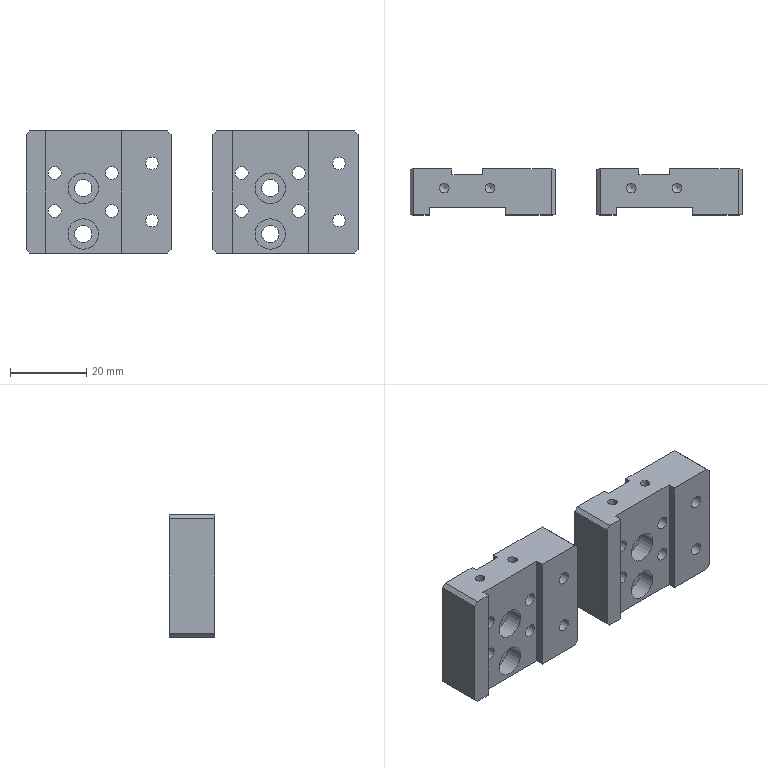Part | 2 solids | 108 faces | box 87 x 12 x 32 mm | volume 19085 mm3 | plane 56 | cylinder 44 | cone 8 | commonest cylinder face diameters 2.5 x8 3.4 x8 6.5 x8 2 x4 3.3 x4 4 x4